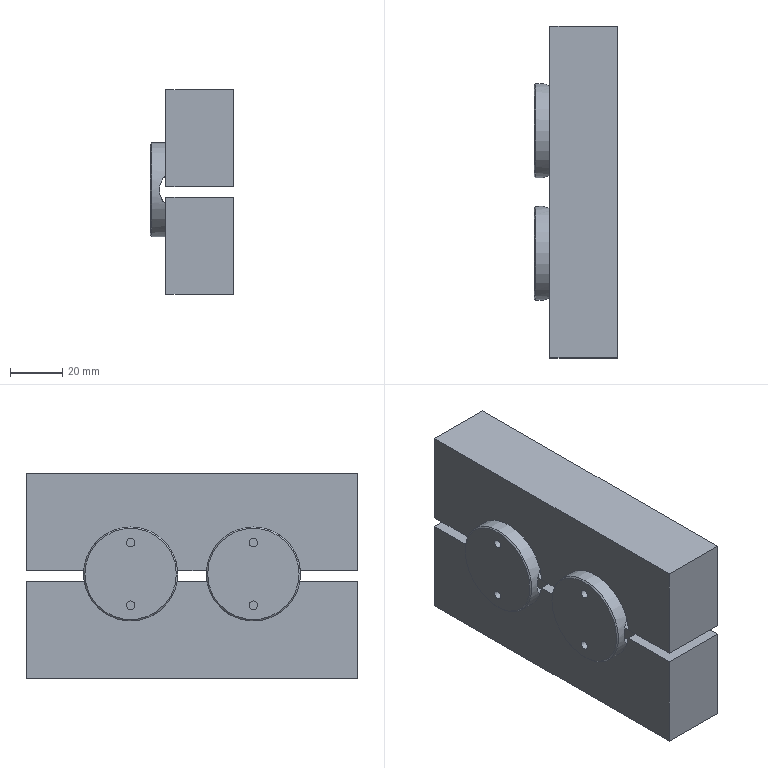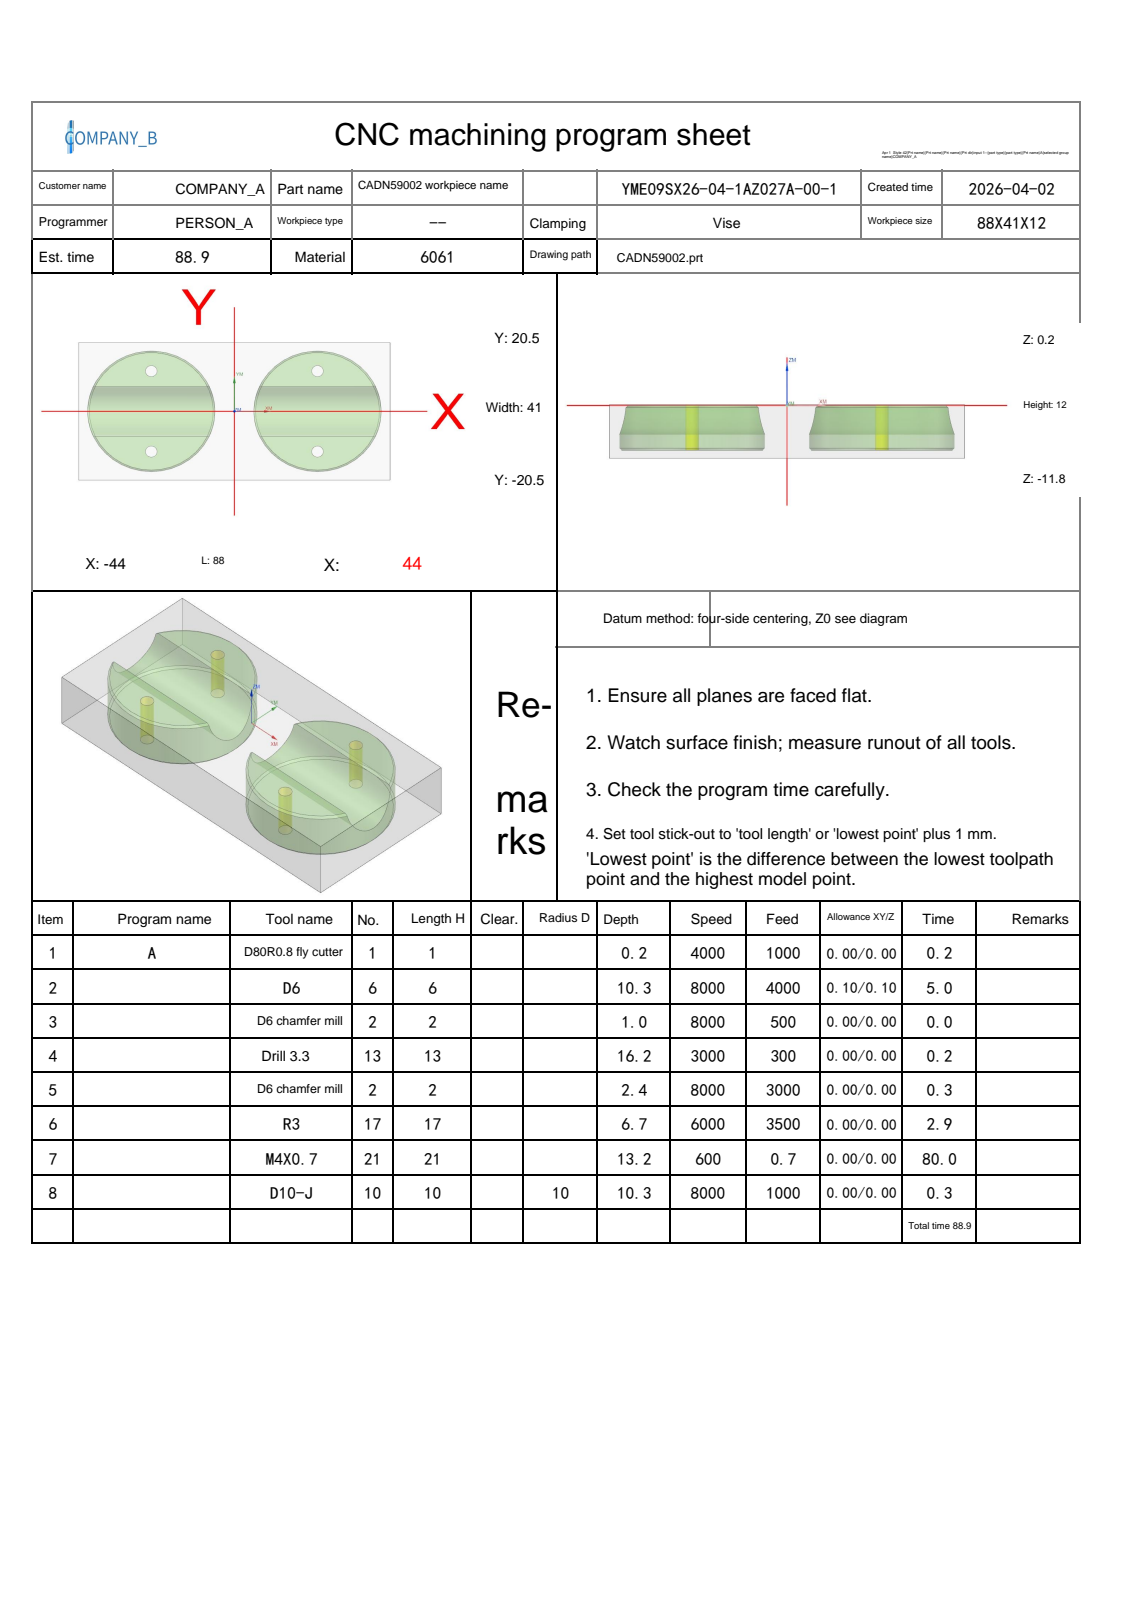NC program | NX | posted by the shop | part box 32 x 127 x 78.432 mm
Lines 6165 to 8369 of 8369:
N3 T02 M06
(D6 chamfer mill  D=6. R=0. H=02 ce=0.00 di=0.10)
G00 G90 G54 X-23.5 Y-12. M03 S8000
G43 H02 Z20.
M08
G98 G81 X-23.5 Y-12. Z-.8 R1. F500.
Y12.
X23.5 Y-12.
Y12.
G80
G00 Z20.
G91 G28 Z0.0
M05
M09
G91 G28 Z0.0
M01
N4 T13 M06
(drill 3.3 D=3.3 DR_a=118 H=13)
G00 G90 G54 X-23.5 Y-12. M03 S3000
G43 H13 Z20.
M08
G98 G83 X-23.5 Y-12. Z-15.991 R1. F300. Q2.
Y12.
X23.5 Y-12.
Y12.
G80
G00 Z20.
G91 G28 Z0.0
M05
M09
G91 G28 Z0.0
M01
N5 T02 M06
(D6 chamfer mill  D=6. R=0. H=02 ce=0.00 di=0.00)
G00 G90 G54 X7.369 Y-6.165 M03 S8000
G43 H02 Z20.
M08
Z2.927
G01 Z-1.499 F3000.
X7.657 Y-6.133
X23.5
X39.343
X39.631 Y-6.165
Z2.927
G00 Z20.
Y6.165
Z2.927
G01 Z-1.499
X39.343 Y6.133
X23.5
X7.657
X7.369 Y6.165
Z2.927
G00 Z20.
X-39.631 Y-6.165
Z2.927
G01 Z-1.499
X-39.343 Y-6.133
X-23.5
X-7.657
X-7.369 Y-6.165
Z2.927
G00 Z20.
Y6.165
Z2.927
G01 Z-1.499
X-7.657 Y6.133
X-23.5
X-39.343
X-39.631 Y6.165
Z2.927
G00 Z20.
G00 G90 X-23.5 Y-12. M03 S8000
Z20.
G98 G81 X-23.5 Y-12. Z-2.2 R3. F500.
Y12.
X23.5 Y-12.
Y12.
G80
G00 Z20.
G00 G90 X-5.262 Y-5.033 M03 S6500
Z20.
Z.3
G01 Z-1.2 F1500.
X-5.284 Y-5.071
X-5.301 Y-5.112
X-6.442 Y-7.662
X-6.452 Y-7.685
X-6.459 Y-7.7
X-6.472 Y-7.73
X-6.491 Y-7.772
X-6.503 Y-7.797
X-6.53 Y-7.856
G02 X-9.998 Y-12.938 I-16.97 J7.856
G01 X-10.106 Y-13.049
G02 X-14.986 Y-16.65 I-13.394 J13.049
X-15.531 Y-16.917 I-8.514 J16.65
X-16.05 Y-17.152 I-7.969 J16.917
X-16.645 Y-17.398 I-7.45 J17.152
X-18.14 Y-17.915 I-6.855 J17.398
X-18.931 Y-18.133 I-5.36 J17.915
G01 X-18.974 Y-18.144
G02 X-19.486 Y-18.264 I-4.526 J18.144
X-19.856 Y-18.342 I-4.014 J18.264
G01 X-19.991 Y-18.368
G02 X-23.5 Y-18.7 I-3.509 J18.368
X-28.05 Y-18.138 I0.0 J18.7
G01 X-28.085 Y-18.129
X-28.15 Y-18.113
X-28.271 Y-18.081
X-28.291 Y-18.076
G02 X-29.664 Y-17.655 I4.791 J18.076
G01 X-29.724 Y-17.634
G02 X-30.114 Y-17.491 I6.224 J17.634
X-30.371 Y-17.392 I6.614 J17.491
G01 X-30.411 Y-17.376
G02 X-31.138 Y-17.069 I6.911 J17.376
G01 X-31.185 Y-17.048
X-31.27 Y-17.01
X-31.308 Y-16.992
X-31.401 Y-16.949
X-31.49 Y-16.907
G02 X-40.436 Y-7.928 I7.99 J16.907
G01 X-40.456 Y-7.885
X-40.487 Y-7.819
X-40.51 Y-7.768
X-40.531 Y-7.723
X-40.548 Y-7.685
X-40.558 Y-7.662
X-40.568 Y-7.639
X-41.198 Y-6.233
X-41.699 Y-5.112
X-41.716 Y-5.071
X-41.738 Y-5.033
Z.3
G00 Z20.
Y5.033
Z.3
G01 Z-1.2
X-41.716 Y5.071
X-41.699 Y5.112
X-40.568 Y7.639
X-40.562 Y7.654
X-40.551 Y7.677
X-40.528 Y7.73
X-40.513 Y7.762
X-40.507 Y7.774
X-40.497 Y7.797
X-40.492 Y7.807
X-40.487 Y7.819
X-40.48 Y7.833
X-40.463 Y7.87
X-40.455 Y7.889
X-40.444 Y7.911
X-40.44 Y7.921
G02 X-40.329 Y8.154 I16.94 J-7.921
X-33.334 Y15.906 I16.829 J-8.154
X-33.121 Y16.035 I9.834 J-15.906
X-32.62 Y16.325 I9.621 J-16.035
G01 X-32.571 Y16.352
X-32.56 Y16.359
X-32.549 Y16.365
X-32.444 Y16.422
G02 X-32.105 Y16.602 I8.944 J-16.422
X-26.473 Y18.462 I8.605 J-16.602
G01 X-26.347 Y18.482
X-26.216 Y18.502
G02 X-25.978 Y18.535 I2.716 J-18.502
G01 X-25.933 Y18.541
X-25.902 Y18.545
G02 X-25.674 Y18.573 I2.402 J-18.545
G01 X-25.66 Y18.575
X-25.613 Y18.58
X-25.415 Y18.602
G02 X-25.014 Y18.639 I1.915 J-18.602
X-24.355 Y18.68 I1.514 J-18.639
G01 X-24.192 Y18.687
X-24.005 Y18.693
X-23.952 Y18.695
X-23.94
X-23.848 Y18.697
X-23.819
X-23.801 Y18.698
G02 X-23.5 Y18.7 I.301 J-18.698
X-22.885 Y18.69 I0.0 J-18.7
X-17.308 Y17.645 I-.615 J-18.69
X-15.815 Y17.048 I-6.192 J-17.645
G01 X-15.785 Y17.034
X-15.748 Y17.017
X-15.599 Y16.949
G02 X-14.745 Y16.524 I-7.901 J-16.949
X-14.015 Y16.116 I-8.755 J-16.524
G01 X-13.997 Y16.105
G02 X-13.493 Y15.797 I-9.503 J-16.105
X-13.265 Y15.65 I-10.007 J-15.797
G01 X-13.256 Y15.644
X-13.244 Y15.637
X-13.231 Y15.628
X-13.157 Y15.579
X-13.141 Y15.569
X-13.013 Y15.482
G02 X-6.57 Y7.942 I-10.487 J-15.482
G01 X-6.564 Y7.928
X-6.551 Y7.9
X-6.533 Y7.862
X-6.528 Y7.851
X-6.523 Y7.841
X-6.503 Y7.797
X-6.487 Y7.762
X-6.476 Y7.738
X-6.471 Y7.726
X-6.466 Y7.715
X-6.456 Y7.693
X-6.452 Y7.684
X-6.432 Y7.64
X-5.301 Y5.112
X-5.284 Y5.071
X-5.261 Y5.033
Z.3
G00 Z20.
X5.262
Z.3
G01 Z-1.2
X5.284 Y5.071
X5.301 Y5.112
X5.802 Y6.233
X6.432 Y7.639
X6.444 Y7.666
X6.449 Y7.677
X6.467 Y7.717
X6.484 Y7.756
X6.503 Y7.798
X6.517 Y7.827
X6.53 Y7.856
X6.539 Y7.876
X6.554 Y7.907
G02 X6.759 Y8.332 I16.946 J-7.907
X6.854 Y8.521 I16.741 J-8.332
G01 X6.876 Y8.563
X6.889 Y8.589
X6.929 Y8.665
G02 X7.564 Y9.784 I16.571 J-8.665
X7.738 Y10.062 I15.936 J-9.784
X8.021 Y10.493 I15.762 J-10.062
X23.5 Y18.7 I15.479 J-10.493
X32.987 Y16.115 I0.0 J-18.7
X33.233 Y15.967 I-9.487 J-16.115
X40.442 Y7.915 I-9.733 J-15.967
G01 X40.449 Y7.901
X40.453 Y7.892
X40.461 Y7.875
X40.468 Y7.861
X40.477 Y7.841
X40.483 Y7.826
X40.495 Y7.8
X40.504 Y7.782
X40.509 Y7.771
X40.536 Y7.712
X40.544 Y7.694
X40.568 Y7.639
X41.699 Y5.112
X41.716 Y5.071
X41.738 Y5.033
Z.3
G00 Z20.
Y-5.033
Z.3
G01 Z-1.2
X41.716 Y-5.071
X41.699 Y-5.112
X40.568 Y-7.639
X40.562 Y-7.655
X40.534 Y-7.715
X40.524 Y-7.739
X40.514 Y-7.76
X40.454 Y-7.89
X40.446 Y-7.907
X40.401 Y-8.003
X40.394 Y-8.018
X40.36 Y-8.089
X40.306 Y-8.2
X40.286 Y-8.242
G02 X40.021 Y-8.761 I-16.786 J8.242
X39.727 Y-9.293 I-16.521 J8.761
X25.965 Y-18.537 I-16.227 J9.293
G01 X25.931 Y-18.541
G02 X25.621 Y-18.579 I-2.431 J18.541
G01 X25.487 Y-18.594
X25.39 Y-18.604
X25.271 Y-18.616
X25.211 Y-18.622
G02 X23.5 Y-18.7 I-1.711 J18.622
X22.897 Y-18.69 I0.0 J18.7
X22.668 Y-18.681 I.603 J18.69
X22.382 Y-18.667 I.832 J18.681
X15.63 Y-16.963 I1.118 J18.667
X15.406 Y-16.858 I7.87 J16.963
X15.059 Y-16.687 I8.094 J16.858
X11.652 Y-14.468 I8.441 J16.687
G01 X11.582 Y-14.41
X11.536 Y-14.372
G02 X11.2 Y-14.086 I11.964 J14.372
X7.649 Y-9.922 I12.3 J14.086
X6.943 Y-8.693 I15.851 J9.922
X6.571 Y-7.943 I16.557 J8.693
G01 X6.551 Y-7.9
X6.544 Y-7.885
X6.481 Y-7.749
X6.432 Y-7.64
X5.301 Y-5.112
X5.284 Y-5.071
X5.261 Y-5.033
Z.3
G00 Z20.
G91 G28 Z0.0
M05
M09
G91 G28 Z0.0
M01
N6 T17 M06
(R3  D=6. R=3. H=17 ce=0.00 di=0.00)
G00 G90 G54 X41.596 Y-4.514 M03 S6000
G43 H17 Z20.
M08
Z2.989
G01 Z-2.299 F3500.
X39.597 Z-2.224
X39.476 Z-2.219
X39.348 Z-2.222
X37.885 Z-2.213
X36.422 Z-2.21
X17.099 Z-2.208
X9.602 Z-2.21
X7.884 Z-2.223
X7.651
X7.523 Z-2.221
X7.381 Z-2.226
X7.255 Y-4.5 Z-2.315
X7.385 Z-2.318
X7.462 Z-2.315
X7.71 Z-2.318
X8.97 Z-2.313
X9.801 Z-2.308
X36.278
X38.229 Z-2.311
X39.348 Z-2.318
X39.537 Z-2.313
X39.614 Z-2.316
X39.745 Z-2.314
X39.888 Y-4.486 Z-2.415
X39.821 Z-2.405
X39.598 Z-2.406
X39.348 Z-2.413
X37.885 Z-2.407
X9.568
X8.105 Z-2.413
X7.651 Z-2.414
X7.179 Z-2.405
X7.115 Z-2.414
X6.98 Y-4.472 Z-2.51
X7.085 Z-2.496
X7.163 Z-2.495
X7.233 Z-2.502
X7.382 Z-2.505
X7.651 Z-2.503
X9.114 Z-2.499
X9.602 Z-2.497
X38.373 Z-2.498
X39.348 Z-2.502
X39.573 Z-2.496
X39.836 Z-2.495
X39.915 Z-2.497
X40.026 Z-2.511
X40.164 Y-4.458 Z-2.607
X40.028 Z-2.589
X39.752 Z-2.584
X39.156 Z-2.589
X37.885 Z-2.586
X9.602
X7.651 Z-2.589
X7.438 Z-2.603
X7.333 Z-2.601
X7.163 Z-2.585
X6.972 Z-2.589
X6.845 Z-2.605
X6.769 Y-4.45 Z-2.659
X6.651 Y-4.444 Z-2.699
X6.676 Z-2.705
X6.858 Z-2.682
X7.163 Z-2.676
X7.325 Z-2.692
X7.448 Z-2.69
X7.651 Z-2.677
X11.54 Z-2.675
X38.373
X39.043 Z-2.677
X39.702 Z-2.674
X40.142 Z-2.682
X40.303 Z-2.703
X40.376 Y-4.432 Z-2.757
X40.381 Y-4.431 Z-2.764
X40.384 Y-4.429 Z-2.775
X40.339 Z-2.784
X39.836 Z-2.775
X39.649 Z-2.771
X7.651 Z-2.772
X7.586 Z-2.776
X7.377
X7.215 Z-2.78
X7.163 Z-2.775
X6.734 Z-2.783
X6.676 Z-2.79
X6.612 Z-2.774
X6.594 Y-4.411 Z-2.87
X6.632 Z-2.88
X6.851 Z-2.879
X7.375 Z-2.869
X39.624
X40.148 Z-2.879
X40.368 Z-2.88
X40.407 Z-2.87
X40.434 Y-4.39 Z-2.973
X40.324 Z-2.971
X39.827
X39.627 Z-2.966
X7.373
X7.142 Z-2.971
X6.676 Z-2.97
X6.568 Z-2.973
X6.543 Y-4.369 Z-3.066
X6.676 Z-3.063
X7.314 Z-3.065
X7.37 Z-3.064
X39.629
X39.836 Z-3.065
X40.324 Z-3.062
X40.458 Z-3.065
X40.482 Y-4.345 Z-3.159
X40.324 Z-3.156
X39.836 Z-3.159
X7.163
X6.676 Z-3.156
X6.518 Z-3.16
X6.5 Y-4.329 Z-3.225
X6.494 Y-4.321 Z-3.251
X6.552 Z-3.252
X6.593 Z-3.244
X6.676 Z-3.242
X7.163 Z-3.246
X39.836
X40.324 Z-3.242
X40.406 Z-3.244
X40.447 Z-3.252
X40.507 Z-3.253
X40.53 Y-4.293 Z-3.343
X40.324 Z-3.337
X39.836 Z-3.34
X7.163
X6.514 Z-3.336
X6.471 Z-3.338
X6.447 Y-4.265 Z-3.431
X6.599 Z-3.423
X7.163 Z-3.427
X39.836
X40.324 Z-3.424
X40.554 Z-3.435
X40.577 Y-4.236 Z-3.523
X40.324 Z-3.511
X39.836 Z-3.514
X7.163
X6.66 Z-3.512
X6.423 Z-3.523
X6.398 Y-4.199 Z-3.613
X6.511 Z-3.607
X6.676 Z-3.604
X7.163 Z-3.607
X39.836
X40.324 Z-3.604
X40.488 Z-3.607
X40.601 Z-3.613
X40.627 Y-4.162 Z-3.702
X40.324 Z-3.696
X39.836 Z-3.698
X6.989 Z-3.697
X6.676 Z-3.696
X6.374 Z-3.702
X6.347 Y-4.127 Z-3.791
X6.676 Z-3.785
X8.184 Z-3.787
X39.836
X40.324 Z-3.785
X40.655 Z-3.791
X40.683 Y-4.087 Z-3.878
X40.453 Z-3.874
X7.034 Z-3.875
X6.547 Z-3.874
X6.319 Z-3.878
X6.29 Y-4.045 Z-3.965
X6.676 Z-3.962
X40.62 Z-3.963
X40.711 Z-3.965
X40.739 Y-4.004 Z-4.051
X6.262
X6.233 Y-3.957 Z-4.137
X40.768 Z-4.136
X40.796 Y-3.911 Z-4.22
X6.204
X6.173 Y-3.864 Z-4.303
X40.324
X40.827
X40.859 Y-3.814 Z-4.384
X40.811 Z-4.38
X39.279 Z-4.382
X6.438 Z-4.381
X6.188
X6.142 Z-4.384
X6.124 Y-3.787 Z-4.428
X6.109 Y-3.761 Z-4.466
X40.301 Z-4.467
X40.891 Z-4.466
X40.923 Y-3.706 Z-4.546
X40.811 Z-4.545
X40.324 Z-4.547
X6.676
X6.077
X6.045 Y-3.652 Z-4.624
X6.188 Z-4.623
X7.727 Z-4.625
X40.324
X40.811 Z-4.623
X40.955 Z-4.624
X40.966 Y-3.634 Z-4.65
X40.988 Y-3.595 Z-4.7
X40.811 Z-4.698
X38.974 Z-4.7
X30.083
X29.924 Z-4.702
X22.928
X22.768 Z-4.699
X6.676 Z-4.7
X6.148 Z-4.698
X6.012 Z-4.7
X5.979 Y-3.536 Z-4.773
X22.768
X23.164 Z-4.78
X29.687
X30.083 Z-4.774
X40.522 Z-4.773
X41.021 Z-4.774
X41.054 Y-3.476 Z-4.848
X30.083
X29.743 Z-4.853
X23.108
X22.768 Z-4.847
X5.945 Z-4.848
X5.911 Y-3.414 Z-4.927
X5.967 Z-4.925
X22.768 Z-4.924
X22.859 Z-4.926
X29.992 Z-4.927
X30.083 Z-4.926
X41.055 Z-4.925
X41.089 Z-4.927
X41.102 Y-3.392 Z-4.956
X41.122 Y-3.352 Z-4.997
X14.234 Z-4.996
X5.878 Z-4.997
X5.844 Y-3.287 Z-5.066
X41.156
X41.19 Y-3.222 Z-5.135
X5.81
X5.776 Y-3.155 Z-5.206
X41.224
X41.259 Y-3.083 Z-5.273
X40.946 Z-5.272
X40.593 Z-5.274
X40.458 Z-5.273
X6.541
X6.188 Z-5.274
X6.053 Z-5.272
X5.741 Z-5.273
X5.706 Y-3.01 Z-5.339
X5.907 Z-5.338
X6.188 Z-5.341
X6.395 Z-5.339
X40.605
X40.886 Z-5.341
X41.092 Z-5.338
X41.294
X41.328 Y-2.939 Z-5.403
X5.829
X5.672
X5.658 Y-2.907 Z-5.433
X5.64 Y-2.867 Z-5.465
X5.7 Z-5.463
X41.299
X41.36 Z-5.465
X41.392 Y-2.794 Z-5.525
X41.299 Z-5.522
X5.7 Z-5.521
X5.608 Z-5.525
X5.575 Y-2.719 Z-5.586
X5.7 Z-5.581
X41.299
X41.425 Z-5.586
X41.449 Y-2.665 Z-5.631
X41.458 Y-2.641 Z-5.646
X41.323 Z-5.64
X5.676
X5.543 Z-5.646
X5.512 Y-2.56 Z-5.7
X5.594 Z-5.696
X41.405
X41.489 Z-5.7
X41.521 Y-2.478 Z-5.753
X41.487 Z-5.751
X5.513
X5.481 Z-5.753
X5.45 Y-2.398 Z-5.806
X5.7 Z-5.804
X41.517
X41.552 Z-5.806
X41.583 Y-2.317 Z-5.859
X41.437 Z-5.853
X5.563
X5.419 Z-5.859
X5.389 Y-2.234 Z-5.907
X5.592 Z-5.905
X5.646 Z-5.903
X41.353 Z-5.902
X41.408 Z-5.905
X41.611 Z-5.907
X41.628 Y-2.18 Z-5.938
X41.637 Y-2.148 Z-5.954
X41.233 Z-5.952
X5.635
X5.361 Z-5.954
X5.336 Y-2.06 Z-5.999
X27.935 Z-5.996
X41.663 Z-5.999
X41.688 Y-1.973 Z-6.042
X20.504 Z-6.039
X5.311 Z-6.043
X5.301 Y-1.938 Z-6.06
X5.287 Y-1.885 Z-6.083
X26.989 Z-6.081
X41.712 Z-6.083
X41.737 Y-1.796 Z-6.121
X12.402
X5.262 Z-6.122
X5.238 Y-1.706 Z-6.16
X41.762
X41.783 Y-1.613 Z-6.196
X41.145 Z-6.199
X40.811 Z-6.197
X6.188
X5.547 Z-6.199
X5.217 Z-6.196
X5.196 Y-1.521 Z-6.231
X5.918 Z-6.233
X6.188 Z-6.231
X40.811
X41.299 Z-6.233
X41.804 Z-6.231
X41.824 Y-1.429 Z-6.264
X5.176
X5.155 Y-1.336 Z-6.294
X5.213 Z-6.293
X20.58
X20.818 Z-6.289
X21.424
X21.543 Z-6.293
X41.787
X41.845 Z-6.294
X41.865 Y-1.242 Z-6.323
X21.731 Z-6.322
X21.518 Z-6.316
X20.818
X20.391 Z-6.322
X7.407 Z-6.323
X5.135
X5.119 Y-1.146 Z-6.349
X20.462 Z-6.348
X20.818 Z-6.343
X21.615
X21.793 Z-6.348
X41.881 Z-6.349
X41.896 Y-1.05 Z-6.373
X26.426 Z-6.372
X21.793
X21.711 Z-6.37
X20.818
X20.655 Z-6.372
X5.104 Z-6.373
X5.089 Y-.954 Z-6.397
X27.157 Z-6.394
X41.787 Z-6.395
X41.911 Z-6.396
X41.925 Y-.857 Z-6.415
X23.275 Z-6.414
X5.075 Z-6.415
X5.06 Y-.759 Z-6.431
X5.213 Z-6.433
X41.819
X41.94 Z-6.431
X41.944 Y-.733 Z-6.435
X41.949 Y-.661 Z-6.447
X41.787 Z-6.449
X5.146
X5.051 Z-6.447
X5.043 Y-.562 Z-6.463
X41.957
X41.965 Y-.463 Z-6.475
X5.035
X5.027 Y-.364 Z-6.485
X5.213 Z-6.483
X41.909
X41.973 Z-6.485
X41.981 Y-.265 Z-6.496
X41.81 Z-6.491
X5.19
X5.019 Z-6.496
X5.017 Y-.242 Z-6.498
Y-.165
X5.213 Z-6.495
X41.864
X41.983 Z-6.498
Y-.065
X5.017
Y.035
X41.983
Y.135 Z-6.497
X41.895 Z-6.495
X5.105 Z-6.496
X5.016 Z-6.498
Y.235
X5.205 Z-6.493
X41.794 Z-6.492
X41.983 Z-6.497
X41.976 Y.334 Z-6.487
X41.787 Z-6.484
X5.12 Z-6.485
X5.023 Z-6.488
X5.031 Y.434 Z-6.477
X15.941 Z-6.474
X29.412 Z-6.477
X41.969 Z-6.476
X41.965 Y.485 Z-6.472
X41.961 Y.533 Z-6.466
X18.867 Z-6.464
X14.966 Z-6.461
X14.869 Z-6.463
X5.039 Z-6.466
X5.046 Y.631 Z-6.451
X6.92 Z-6.452
X14.67 Z-6.45
X14.966 Z-6.445
X18.719 Z-6.446
X18.867 Z-6.449
X32.521 Z-6.45
X41.883 Z-6.452
X41.953 Z-6.45
X41.946 Y.73 Z-6.435
X41.787 Z-6.438
X24.956 Z-6.432
X18.861 Z-6.434
X18.62 Z-6.43
X14.966 Z-6.429
X14.478 Z-6.437
X5.694 Z-6.438
X5.21
X5.054 Z-6.435
X5.068 Y.828 Z-6.42
X14.682 Z-6.418
X14.966 Z-6.413
X18.521 Z-6.414
X18.663 Z-6.416
X34.02 Z-6.418
X41.931 Z-6.42
X41.917 Y.926 Z-6.403
X14.966 Z-6.397
X5.299 Z-6.402
X5.083 Z-6.403
X5.089 Y.969 Z-6.395
X5.097 Y1.024 Z-6.381
X17.16 Z-6.378
X23.256 Z-6.379
X23.311 Z-6.377
X41.902 Z-6.381
X41.888 Y1.12 Z-6.356
X29.899 Z-6.354
X29.595 Z-6.351
X23.408
X23.256 Z-6.355
X5.112 Z-6.356
X5.126 Y1.216 Z-6.331
X23.266
X23.505 Z-6.324
X29.595 Z-6.325
X30.073 Z-6.329
X41.792 Z-6.332
X41.874 Z-6.33
X41.853 Y1.312 Z-6.303
X41.787 Z-6.302
X29.881 Z-6.3
X29.595 Z-6.298
X23.601 Z-6.297
X23.458 Z-6.302
X5.213
X5.147 Z-6.303
X5.168 Y1.407 Z-6.273
X23.65 Z-6.272
X23.697 Z-6.271
X41.832 Z-6.273
X41.821 Y1.454 Z-6.259
X41.81 Y1.502 Z-6.24
X5.407 Z-6.241
X5.19 Z-6.24
X5.211 Y1.595 Z-6.204
X5.783 Z-6.207
X5.985 Z-6.204
X40.811
X41.378 Z-6.206
X41.789 Z-6.204
X41.768 Y1.688 Z-6.168
X5.232
X5.256 Y1.779 Z-6.128
X41.744
X41.718 Y1.871 Z-6.088
X5.282
X5.307 Y1.962 Z-6.047
X41.692 Z-6.046
X41.666 Y2.051 Z-6.002
X5.333
X5.359 Y2.14 Z-5.957
X5.7 Z-5.955
X41.381
X41.64 Z-5.957
X41.622 Y2.201 Z-5.925
X41.613 Y2.227 Z-5.91
X41.299 Z-5.906
X5.7
X5.385 Z-5.91
X5.417 Y2.313 Z-5.861
X5.7 Z-5.855
X41.299
X41.585 Z-5.861
X41.553 Y2.399 Z-5.81
X41.299 Z-5.804
X5.7
X5.45 Z-5.81
X5.459 Y2.423 Z-5.795
X5.482 Y2.482 Z-5.754
X5.7 Z-5.749
X41.299
X41.52 Z-5.754
X41.487 Y2.564 Z-5.696
X41.299 Z-5.692
X5.7
X5.514 Z-5.696
X5.546 Y2.646 Z-5.641
X5.7 Z-5.635
X41.336 Z-5.636
X41.455 Z-5.641
X41.448 Y2.665 Z-5.629
X41.422 Y2.726 Z-5.579
X41.299 Z-5.574
X5.7
X5.579 Z-5.579
X5.613 Y2.804 Z-5.515
X5.7 Z-5.512
X41.299
X41.387 Z-5.515
X41.353 Y2.883 Z-5.452
X41.299 Z-5.451
X5.7 Z-5.45
X5.647 Z-5.452
X5.67 Y2.935 Z-5.407
X5.681 Y2.958 Z-5.386
X5.803 Z-5.385
X6.188 Z-5.387
X6.29 Z-5.386
X40.709
X40.811 Z-5.388
X41.095 Z-5.387
X41.299 Z-5.385
X41.319 Z-5.386
X41.284 Y3.031 Z-5.319
X41.049
X40.8 Z-5.323
X40.562 Z-5.32
X6.438
X6.188 Z-5.323
X5.95 Z-5.319
X5.716
X5.751 Y3.104 Z-5.253
X6.097
X6.493 Z-5.255
X6.584 Z-5.254
X40.415
X40.811 Z-5.255
X40.903 Z-5.253
X41.249
X41.228 Y3.15 Z-5.213
X41.215 Y3.175 Z-5.186
X5.785
X5.82 Y3.243 Z-5.115
X5.999
X6.188 Z-5.111
X40.811 Y3.244 Z-5.112
X41. Z-5.115
X41.18
X41.145 Y3.312 Z-5.044
X40.811 Z-5.038
X6.188
X5.855 Z-5.044
X5.891 Y3.38 Z-4.971
X6.188 Z-4.965
X10.882 Z-4.967
X40.324
X40.811 Z-4.965
X41.109 Z-4.97
X41.074 Y3.443 Z-4.893
X40.811 Z-4.889
X30.571
X30.365 Z-4.892
X16.147
X15.941 Z-4.89
X6.676
X6.188 Z-4.889
X5.926 Z-4.893
X5.961 Y3.505 Z-4.816
X6.188 Z-4.811
X15.941 Z-4.813
X16.397 Z-4.818
X30.114
X30.571 Z-4.811
X40.811 Z-4.812
X41.039 Z-4.816
X41.005 Y3.566 Z-4.742
X40.949 Z-4.739
X40.811 Z-4.736
X30.571 Z-4.734
X30.296 Z-4.738
X16.216 Z-4.74
X15.941 Z-4.737
X6.188 Z-4.736
X6.051 Z-4.739
X5.994 Z-4.742
X6.027 Y3.626 Z-4.67
X6.188 Z-4.661
X18.404 Z-4.662
X31.042 Z-4.658
X40.828 Z-4.662
X40.973 Z-4.67
X40.94 Y3.682 Z-4.59
X40.811 Z-4.583
X24.04 Z-4.582
X22.472
X22.281 Z-4.577
X16.429 Z-4.579
X16.238 Z-4.583
X6.188
X6.061 Z-4.59
X6.092 Y3.736 Z-4.51
X6.188 Z-4.504
X16.017 Z-4.503
X16.429 Z-4.496
X22.281 Z-4.494
X22.692 Z-4.505
X40.811 Z-4.504
X40.908 Z-4.51
X40.897 Y3.755 Z-4.485
X40.875 Y3.79 Z-4.425
X40.811 Z-4.42
X22.628 Z-4.421
X22.281 Z-4.412
X16.429 Z-4.413
X16.082 Z-4.42
X6.188
X6.125 Z-4.425
X6.159 Y3.842 Z-4.337
X6.188 Z-4.335
X9.114 Z-4.336
X16.292
X16.429 Z-4.333
X22.281
X22.417 Z-4.337
X40.46 Z-4.336
X40.811 Z-4.335
X40.842 Z-4.337
X40.809 Y3.893 Z-4.249
X37.4 Z-4.251
X6.676 Z-4.25
X6.192 Z-4.249
X6.222 Y3.941 Z-4.162
X40.324 Z-4.163
X40.778 Z-4.162
X40.749 Y3.989 Z-4.076
X6.252
X6.282 Y4.033 Z-3.987
X7.02 Z-3.986
X39.979
X40.719 Z-3.987
X40.69 Y4.076 Z-3.899
X40.496 Z-3.895
X30.647 Z-3.896
X7.163
X6.504 Z-3.895
X6.311 Z-3.898
X6.34 Y4.119 Z-3.81
X6.674 Z-3.804
X7.163 Z-3.806
X39.835
X40.324 Z-3.804
X40.661 Z-3.81
X40.632 Y4.156 Z-3.717
X40.324 Z-3.712
X39.836 Z-3.714
X32.034
X31.734 Z-3.718
X31.358
X31.058 Z-3.714
X7.163
X6.676 Z-3.712
X6.369 Z-3.717
X6.395 Y4.193 Z-3.627
X6.487 Z-3.622
X6.676 Z-3.619
X7.163 Z-3.621
X31.058
X31.436 Z-3.627
X31.656
X32.034 Z-3.621
X39.836
X40.324 Z-3.619
X40.512 Z-3.622
X40.605 Z-3.627
X40.581 Y4.229 Z-3.541
X40.324 Z-3.53
X39.836 Z-3.532
X32.034
X31.149 Z-3.534
X31.058 Z-3.533
X7.163
X6.63 Z-3.531
X6.419 Z-3.541
X6.426 Y4.24 Z-3.514
X6.443 Y4.26 Z-3.453
X6.676 Z-3.442
X7.651 Z-3.444
X23.096 Z-3.441
X31.386 Z-3.443
X31.466 Z-3.439
X36.422
X36.582 Z-3.444
X39.836 Z-3.445
X40.324 Z-3.442
X40.558 Z-3.454
X40.535 Y4.288 Z-3.366
X40.426 Z-3.363
X40.324 Z-3.359
X39.836 Z-3.361
X36.808
X36.422 Z-3.347
X31.353
X31.161 Z-3.357
X20.33 Z-3.351
X7.163 Z-3.36
X6.676 Z-3.359
X6.573 Z-3.363
X6.466 Z-3.366
X6.489 Y4.315 Z-3.277
X6.586 Z-3.275
X6.616 Z-3.269
X6.676 Z-3.267
X7.163 Z-3.269
X21.425 Z-3.26
X31.058 Z-3.265
X31.242 Z-3.256
X36.422
X36.79 Z-3.269
X39.836
X40.324 Z-3.267
X40.383 Z-3.269
X40.413 Z-3.275
X40.511 Z-3.277
X40.499 Y4.33 Z-3.231
X40.487 Y4.341 Z-3.18
X40.324 Z-3.176
X39.836 Z-3.178
X36.584
X36.422 Z-3.172
X31.139
X31.058 Z-3.176
X17.892 Z-3.174
X7.163 Z-3.178
X6.676 Z-3.176
X6.514 Z-3.18
X6.539 Y4.366 Z-3.084
X6.76 Z-3.08
X7.37 Z-3.081
X39.836 Z-3.082
X40.324 Z-3.08
X40.462 Z-3.084
X40.438 Y4.387 Z-2.99
X40.324 Z-2.988
X39.805 Z-2.986
X39.627 Z-2.983
X7.372
X7.194 Z-2.986
X6.676 Z-2.988
X6.562 Z-2.991
X6.583 Y4.407 Z-2.892
X6.616 Z-2.899
X7.163 Z-2.892
X7.375 Z-2.888
X39.625
X40.083 Z-2.896
X40.384 Z-2.899
X40.413 Z-2.892
X40.39 Y4.425 Z-2.797
X40.324 Z-2.812
X40.297 Z-2.809
X39.836 Z-2.801
X39.813 Z-2.803
X39.623 Z-2.799
X39.378
X39.348 Z-2.797
X7.365 Z-2.796
X6.687 Z-2.809
X6.657 Z-2.807
X6.605 Z-2.797
X6.622 Y4.44 Z-2.716
X6.662 Z-2.724
X6.69 Z-2.725
X6.825 Z-2.708
X7.311 Z-2.699
X8.139 Z-2.701
X37.398 Z-2.7
X39.348 Z-2.702
X39.515 Z-2.712
X39.703 Z-2.714
X39.836 Z-2.702
X40.174 Z-2.708
X40.296 Z-2.723
X40.162 Y4.456 Z-2.621
X40.05 Z-2.607
X39.836 Z-2.603
X39.646 Z-2.621
X39.587 Z-2.622
X39.348 Z-2.607
X36.476 Z-2.603
X8.626 Y4.455 Z-2.604
X7.866 Z-2.606
X7.257 Z-2.601
X6.949 Z-2.607
X6.805 Z-2.626
X6.945 Y4.47 Z-2.529
X7.063 Z-2.513
X7.207 Z-2.511
X7.438 Z-2.512
X7.651 Z-2.518
X9.114 Z-2.513
X37.398
X38.861 Z-2.518
X39.348
X39.618 Z-2.522
X39.747 Z-2.52
X39.836 Z-2.511
X39.936 Z-2.513
X40.033 Z-2.525
X39.897 Y4.484 Z-2.428
X39.829 Z-2.419
X39.348 Z-2.428
X38.367 Z-2.426
X37.376 Z-2.422
X9.108
X7.651 Z-2.428
X7.38 Z-2.421
X7.17 Z-2.419
X7.088 Z-2.431
X7.235 Y4.498 Z-2.328
X7.385 Z-2.329
X7.452 Z-2.327
X7.651 Z-2.333
X9.114 Z-2.325
X15.945 Z-2.322
X37.398 Z-2.324
X38.987 Z-2.333
X39.348
X39.547 Z-2.329
X39.614 Z-2.332
X39.759 Z-2.329
X39.634 Y4.512 Z-2.24
X39.486 Z-2.235
X39.348 Z-2.238
X38.61 Z-2.235
X37.16 Z-2.225
X25.088 Z-2.223
X10.326 Z-2.225
X9.602 Z-2.226
X8.863 Z-2.229
X7.651 Z-2.237
X7.513 Z-2.234
X7.382 Z-2.239
X7.489 Y4.518 Z-2.192
X7.563 Y4.522 Z-2.166
X7.651 Y4.524 Z-2.153
X7.799 Z-2.149
X9.253 Y4.525 Z-2.131
X9.95 Z-2.127
X17.97 Z-2.124
X35.587 Z-2.126
X37.398 Z-2.128
X37.979 Z-2.133
X39.979 Z-2.152
Z2.989
G00 Z20.
X-41.593 Y4.514
Z2.989
G01 Z-2.296
X-39.595 Z-2.22
X-39.475 Z-2.215
X-39.349 Z-2.219
X-37.886 Z-2.209
X-36.423 Z-2.206
X-17.335
X-9.602 Z-2.209
X-7.883 Z-2.222
X-7.652
X-7.524 Z-2.22
X-7.383 Z-2.225
X-7.256 Y4.5 Z-2.314
X-7.386 Z-2.317
X-7.463 Z-2.314
X-7.652 Z-2.317
X-8.482 Z-2.315
X-9.747 Z-2.307
X-36.275 Z-2.304
X-38.226 Y4.501 Z-2.307
X-39.349 Z-2.314
X-39.536 Z-2.309
X-39.615 Z-2.312
X-39.739 Z-2.311
X-39.882 Y4.487 Z-2.411
X-39.819 Z-2.401
X-39.597 Z-2.403
X-39.349 Z-2.409
X-37.886 Z-2.403
X-9.568 Y4.486 Z-2.405
X-8.105 Z-2.412
X-7.652
X-7.18 Z-2.404
X-7.114 Z-2.413
X-6.977 Y4.472 Z-2.509
X-7.086 Z-2.495
X-7.164 Z-2.494
X-7.234 Z-2.501
X-7.383 Z-2.504
X-7.652 Z-2.502
X-9.193 Z-2.498
X-9.602 Z-2.496
X-38.299 Y4.473 Z-2.495
X-39.349 Z-2.499
X-39.618 Z-2.493
X-39.837 Z-2.492
X-39.912 Z-2.493
X-40.02 Z-2.507
X-40.159 Y4.459 Z-2.603
X-40.025 Z-2.585
X-39.755 Z-2.58
X-39.514 Z-2.582
X-39.349 Z-2.586
X-37.886 Z-2.582
X-9.602 Y4.458 Z-2.585
X-8.139 Z-2.589
X-7.652
X-7.439 Z-2.602
X-7.334 Z-2.6
X-7.164 Z-2.584
X-6.973 Z-2.588
X-6.839 Z-2.605
X-6.711 Y4.448 Z-2.676
X-6.893 Z-2.653
X-7.164 Z-2.648
X-7.356 Y4.449 Z-2.666
X-7.41
X-7.652 Z-2.65
X-10.307 Z-2.647
X-38.374 Z-2.645
X-39.349 Z-2.647
X-39.47 Z-2.644
X-39.72 Z-2.643
X-40.104 Z-2.65
X-40.258 Z-2.671
X-40.324 Y4.442 Z-2.719
X-40.356 Y4.436 Z-2.743
X-40.324 Z-2.75
X-40.207 Z-2.734
X-39.675 Z-2.724
X-39.413 Z-2.725
X-39.349 Z-2.726
X-30.815
X-8.253 Z-2.729
X-7.652
X-7.525 Z-2.737
X-7.378
X-7.265 Z-2.74
X-7.164 Z-2.73
X-6.79 Z-2.737
X-6.692 Z-2.749
X-6.661 Z-2.747
X-6.619 Z-2.738
X-6.603 Y4.42 Z-2.821
X-6.67 Z-2.837
X-7.377 Z-2.824
X-39.624 Y4.421 Z-2.822
X-40.328 Z-2.835
X-40.395 Z-2.82
X-40.422 Y4.4 Z-2.927
X-40.411 Z-2.93
X-40.324 Z-2.928
X-39.977 Z-2.926
X-39.626 Z-2.92
X-7.374 Z-2.922
X-7.03 Z-2.928
X-6.674 Z-2.929
X-6.588 Z-2.931
X-6.58 Z-2.93
X-6.554 Y4.379 Z-3.025
X-6.676 Z-3.022
X-7.247 Z-3.021
X-7.372 Z-3.019
X-39.629 Y4.38 Z-3.018
X-39.837 Z-3.02
X-40.324
X-40.446 Z-3.023
X-40.47 Y4.358 Z-3.117
X-40.324 Z-3.113
X-39.837 Z-3.115
X-7.14 Z-3.117
X-6.676 Z-3.115
X-6.53 Z-3.118
X-6.506 Y4.334 Z-3.212
X-6.543 Z-3.205
X-6.676 Z-3.202
X-7.164 Z-3.204
X-10.357
X-10.578 Z-3.196
X-15.454
X-15.674 Z-3.201
X-28.402 Z-3.198
X-39.837 Z-3.202
X-40.324 Z-3.2
X-40.46 Z-3.204
X-40.494 Z-3.211
X-40.505 Y4.323 Z-3.253
X-40.518 Y4.308 Z-3.301
X-40.369 Z-3.298
X-40.354 Z-3.295
X-38.352
X-26.67 Z-3.286
X-17.484 Y4.307 Z-3.291
X-15.885 Z-3.293
X-15.454 Z-3.282
X-10.578
X-10.146 Z-3.298
X-7.164
X-6.649 Z-3.296
X-6.635 Z-3.299
X-6.483 Z-3.303
X-6.459 Y4.279 Z-3.395
X-6.676 Z-3.386
X-7.164 Z-3.388
X-10.265
X-10.578 Z-3.376
X-15.454
X-15.767 Z-3.384
X-26.67 Z-3.379
X-40.009 Z-3.386
X-40.324 Z-3.384
X-40.542 Z-3.394
X-40.566 Y4.25 Z-3.483
X-40.324 Z-3.472
X-39.837 Z-3.474
X-19.395 Z-3.473
X-15.532 Z-3.474
X-15.454 Z-3.472
X-10.578
X-10.5 Z-3.475
X-7.164
X-6.676 Z-3.473
X-6.434 Z-3.485
X-6.427 Y4.24 Z-3.514
X-6.41 Y4.216 Z-3.571
X-6.58 Z-3.563
X-6.676 Z-3.561
X-7.164 Z-3.564
X-14.966 Z-3.563
X-15.157 Z-3.566
X-15.751
X-15.942 Z-3.563
X-39.837
X-40.324 Z-3.56
X-40.419 Z-3.562
X-40.589 Z-3.57
X-40.614 Y4.181 Z-3.656
X-40.562 Z-3.654
X-40.324 Z-3.649
X-39.837 Z-3.652
X-15.942
X-15.444 Z-3.66
X-14.966 Z-3.652
X-6.916 Y4.18 Z-3.651
X-6.676 Z-3.65
X-6.437 Z-3.655
X-6.386 Z-3.657
X-6.361 Y4.144 Z-3.746
X-6.676 Z-3.741
X-7.164 Z-3.743
X-14.966 Z-3.742
X-15.173 Z-3.746
X-15.735
X-15.942 Z-3.743
X-39.837 Y4.145 Z-3.742
X-40.324 Z-3.74
X-40.641 Z-3.745
X-40.661 Y4.119 Z-3.811
X-40.669 Y4.107 Z-3.834
X-40.279 Z-3.829
X-39.837 Z-3.83
X-7.164 Z-3.831
X-6.629 Z-3.829
X-6.332 Z-3.835
X-6.303 Y4.065 Z-3.921
X-6.461 Z-3.918
X-40.11 Y4.066 Z-3.917
X-40.538
X-40.697 Z-3.92
X-40.726 Y4.024 Z-4.006
X-6.275 Y4.023 Z-4.007
X-6.257 Y3.998 Z-4.061
X-6.246 Y3.98 Z-4.092
X-40.754 Y3.981
X-40.782 Y3.934 Z-4.176
X-6.676 Z-4.177
X-6.218 Z-4.176
X-6.188 Y3.887 Z-4.26
X-9.206 Z-4.261
X-40.324 Y3.888 Z-4.26
X-40.812 Z-4.259
X-40.844 Y3.838 Z-4.344
X-40.812 Z-4.342
X-37.154 Z-4.343
X-30.725
X-30.571 Z-4.34
X-24.719 Z-4.339
X-24.565 Z-4.343
X-6.521
X-6.189 Z-4.342
X-6.156 Z-4.345
X-6.125 Y3.789 Z-4.427
X-6.189 Z-4.421
X-24.37 Y3.79 Z-4.422
X-24.719 Z-4.413
X-30.571 Z-4.414
X-30.92 Z-4.42
X-40.812 Z-4.421
X-40.875 Z-4.426
X-40.897 Y3.755 Z-4.485
X-40.906 Y3.739 Z-4.506
X-40.812 Z-4.5
X-30.994 Z-4.499
X-30.571 Z-4.491
X-24.719 Z-4.49
X-24.297 Z-4.501
X-6.189
X-6.094 Z-4.507
X-6.062 Y3.685 Z-4.585
X-6.189 Z-4.578
X-23.154 Z-4.577
X-24.514
X-24.719 Z-4.572
X-30.571 Z-4.574
X-30.777 Z-4.578
X-40.812 Z-4.577
X-40.937 Z-4.584
X-40.97 Y3.63 Z-4.664
X-40.804 Z-4.656
X-28.483
X-16.429 Z-4.653
X-6.18 Z-4.657
X-6.029 Z-4.665
X-5.996 Y3.57 Z-4.737
X-6.059 Z-4.734
X-6.189 Z-4.731
X-16.429 Z-4.729
X-16.688 Z-4.733
X-30.801 Z-4.735
X-31.059 Z-4.732
X-40.812 Z-4.731
X-40.941 Z-4.733
X-41.003 Z-4.737
X-41.036 Y3.51 Z-4.81
X-40.812 Z-4.806
X-31.059 Z-4.807
X-30.585 Z-4.812
X-16.902 Y3.509 Z-4.813
X-16.429 Z-4.805
X-6.189 Z-4.806
X-5.963 Z-4.81
X-5.928 Y3.447 Z-4.888
X-6.189 Z-4.884
X-16.429
X-16.653 Z-4.887
X-30.835 Y3.448
X-31.059 Z-4.884
X-40.324
X-40.812 Z-4.883
X-41.071 Z-4.888
X-41.105 Y3.387 Z-4.963
X-40.812 Z-4.957
X-37.16 Z-4.959
X-6.666
X-6.189 Z-4.958
X-5.894 Z-4.963
X-5.861 Y3.323 Z-5.032
X-6.189 Z-5.026
X-40.812
X-41.139 Z-5.032
X-41.174 Y3.255 Z-5.103
X-41.024
X-40.812 Z-5.099
X-6.189 Z-5.1
X-5.977 Z-5.103
X-5.826
X-5.791 Y3.187 Z-5.174
X-6.676 Z-5.173
X-40.812 Z-5.172
X-41.209 Z-5.173
X-41.228 Y3.15 Z-5.213
X-41.242 Y3.12 Z-5.239
X-6.189 Z-5.24
X-5.758
X-5.725 Y3.05 Z-5.303
X-5.987
X-6.273 Z-5.306
X-6.475 Z-5.303
X-40.525
X-40.812 Z-5.306
X-41.013 Z-5.302
X-41.275
X-41.309 Y2.979 Z-5.366
X-41.155
X-41.01 Z-5.369
X-40.812
X-40.667 Z-5.367
X-6.332
X-6.189 Z-5.369
X-5.989
X-5.845 Z-5.367
X-5.691
X-5.658 Y2.908 Z-5.432
X-5.7 Z-5.431
X-41.298 Z-5.43
X-41.342 Z-5.431
X-41.374 Y2.834 Z-5.491
X-41.3 Z-5.488
X-5.701 Z-5.489
X-5.626 Z-5.491
X-5.593 Y2.758 Z-5.552
X-5.701 Z-5.548
X-41.3 Y2.759
X-41.407 Z-5.551
X-41.44 Y2.684 Z-5.614
X-41.3 Z-5.607
X-5.683 Y2.683 Z-5.608
X-5.56 Z-5.614
X-5.553 Y2.665 Z-5.629
X-5.53 Y2.605 Z-5.668
X-5.701 Z-5.663
X-41.3 Y2.606
X-41.471 Z-5.668
X-41.503 Y2.524 Z-5.724
X-41.3 Z-5.719
X-5.701 Z-5.72
X-5.498 Z-5.724
X-5.467 Y2.444 Z-5.78
X-5.701 Z-5.775
X-41.3
X-41.535 Z-5.78
X-41.544 Y2.423 Z-5.795
X-41.566 Y2.364 Z-5.831
X-41.3 Z-5.825
X-5.701 Y2.363
X-5.436 Z-5.831
X-5.405 Y2.281 Z-5.879
X-5.701 Z-5.874
X-41.3
X-41.595 Z-5.879
X-41.623 Y2.197 Z-5.927
X-41.3 Z-5.924
X-5.669 Y2.196 Z-5.925
X-5.375 Z-5.927
X-5.35 Y2.11 Z-5.972
X-5.701 Z-5.97
X-41.442
X-41.649 Z-5.972
X-41.674 Y2.022 Z-6.016
X-5.325
X-5.3 Y1.934 Z-6.06
X-41.7 Y1.935
X-41.725 Y1.846 Z-6.099
X-5.275
X-5.25 Y1.756 Z-6.139
X-41.75 Y1.757 Z-6.138
X-41.768 Y1.691 Z-6.167
X-41.773 Y1.666 Z-6.177
X-32.201
X-5.335 Z-6.178
X-5.227 Z-6.177
X-5.206 Y1.574 Z-6.212
X-5.698 Z-6.215
X-6.189 Z-6.212
X-41.056
X-41.3 Y1.575 Z-6.215
X-41.794 Z-6.212
X-41.815 Y1.483 Z-6.247
X-5.185 Y1.482
X-5.179 Y1.454 Z-6.259
X-5.164 Y1.39 Z-6.279
X-5.701 Z-6.278
X-23.321 Z-6.276
X-23.385 Z-6.278
X-41.787 Z-6.277
X-41.836 Z-6.279
X-41.856 Y1.297 Z-6.308
X-41.787 Z-6.306
X-23.572
X-23.414 Z-6.302
X-17.405
X-17.089 Z-6.305
X-5.213 Z-6.306
X-5.144 Z-6.308
X-5.124 Y1.202 Z-6.334
X-8.383 Z-6.335
X-16.937 Z-6.333
X-17.405 Z-6.329
X-23.51 Z-6.328
X-23.744 Z-6.335
X-41.876 Z-6.334
X-41.89 Y1.106 Z-6.36
X-25.695 Z-6.358
X-23.744 Z-6.359
X-23.607 Z-6.354
X-17.405 Z-6.355
X-17.13 Z-6.358
X-5.11 Z-6.36
X-5.095 Y1.01 Z-6.384
X-34.067 Z-6.381
X-41.905 Z-6.384
X-41.911 Y.969 Z-6.395
X-41.919 Y.913 Z-6.405
X-32.147 Z-6.401
X-32.034 Z-6.4
X-5.081 Z-6.405
X-5.067 Y.815 Z-6.422
X-25.695 Y.816 Z-6.418
X-28.311 Z-6.419
X-28.466 Z-6.416
X-32.034 Z-6.415
X-32.343 Z-6.42
X-41.933 Z-6.422
X-41.947 Y.718 Z-6.437
X-41.794 Z-6.44
X-33.483 Y.717 Z-6.439
X-32.503 Z-6.438
X-32.034 Z-6.431
X-28.367 Z-6.432
X-28.133 Z-6.436
X-18.38 Z-6.434
X-5.204 Z-6.44
X-5.053 Z-6.437
X-5.046 Y.619 Z-6.452
X-7.042 Z-6.454
X-22.986 Z-6.45
X-28.133 Z-6.451
X-28.268 Z-6.449
X-32.034 Z-6.447
X-32.305 Z-6.451
X-41.896 Z-6.454
X-41.955 Z-6.453
X-41.962 Y.52 Z-6.467
X-30.048 Z-6.464
X-21.794 Z-6.467
X-5.038
X-5.035 Y.485 Z-6.472
X-5.03 Y.421 Z-6.477
X-28.743 Z-6.476
X-38.13 Z-6.477
X-41.97 Z-6.478
X-41.978 Y.322 Z-6.489
X-41.787 Z-6.486
X-5.133 Z-6.485
X-5.023 Z-6.488
X-5.017 Y.242 Z-6.497
Y.222
X-5.193 Z-6.492
X-41.803 Y.223 Z-6.493
X-41.984 Z-6.498
Y.123
X-41.787 Z-6.496
X-5.093 Y.122 Z-6.495
X-5.017 Z-6.497
Y.023 Z-6.498
X-41.983 Z-6.499
Y-.077 Z-6.498
X-5.017
Y-.177
X-5.148 Z-6.494
X-41.853 Z-6.495
X-41.983 Z-6.498
Y-.245
X-41.98 Y-.277 Z-6.494
X-41.822 Z-6.49
X-5.178
X-5.02 Z-6.494
X-5.028 Y-.377 Z-6.484
X-5.213 Z-6.482
X-41.922 Y-.376
X-41.972 Z-6.484
X-41.964 Y-.476 Z-6.474
X-5.036
X-5.044 Y-.575 Z-6.461
X-41.956
X-41.948 Y-.674 Z-6.445
X-41.841 Z-6.447
X-5.16
X-5.052 Z-6.445
X-5.056 Y-.733 Z-6.435
X-5.062 Y-.773 Z-6.429
X-5.213 Z-6.431
X-41.833 Y-.772
X-41.938 Z-6.429
X-41.923 Y-.87 Z-6.413
X-8.81 Y-.871 Z-6.412
X-5.077 Z-6.413
X-5.092 Y-.969 Z-6.394
X-19.415 Y-.968 Z-6.391
X-35.812 Z-6.393
X-41.908 Z-6.394
X-41.894 Y-1.064 Z-6.37
X-26.375 Y-1.065 Z-6.369
X-26.182 Z-6.366
X-25.303
X-25.207 Z-6.369
X-5.213
X-5.106 Z-6.37
X-5.121 Y-1.161 Z-6.344
X-25.207 Z-6.345
X-25.4 Z-6.339
X-26.182
X-26.568 Z-6.344
X-41.879 Z-6.345
X-41.87 Y-1.222 Z-6.328
X-41.862 Y-1.257 Z-6.319
X-28.133 Z-6.317
X-26.578
X-26.182 Z-6.312
X-25.497
X-25.299 Z-6.318
X-5.213
X-5.138 Z-6.319
X-5.159 Y-1.353 Z-6.289
X-5.213 Z-6.287
X-25.491 Y-1.352 Z-6.288
X-25.593 Z-6.285
X-26.182
X-26.386 Z-6.288
X-41.787 Z-6.287
X-41.841 Z-6.289
X-41.82 Y-1.447 Z-6.258
X-5.18 Y-1.448
X-5.201 Y-1.542 Z-6.223
X-5.834 Z-6.226
X-6.189 Z-6.223
X-40.812 Y-1.541
X-41.435 Z-6.226
X-41.799 Z-6.223
X-41.778 Y-1.635 Z-6.188
X-41.059 Z-6.19
X-40.812 Z-6.188
X-6.189
X-5.701 Z-6.19
X-5.222 Z-6.187
X-5.244 Y-1.727 Z-6.151
X-41.757
X-41.731 Y-1.818 Z-6.112
X-14.692 Z-6.111
X-5.269 Y-1.819 Z-6.112
X-5.294 Y-1.91 Z-6.073
X-27.222 Y-1.909 Z-6.07
X-41.706 Z-6.073
X-41.698 Y-1.938 Z-6.06
X-41.68 Y-1.999 Z-6.029
X-19.294 Z-6.026
X-5.319 Z-6.029
X-5.344 Y-2.088 Z-5.984
X-6.189 Z-5.983
X-34.078
X-41.486
X-41.654 Z-5.984
X-41.629 Y-2.177 Z-5.94
X-41.3 Z-5.937
X-5.694
X-5.369 Z-5.939
X-5.376 Y-2.201 Z-5.926
X-5.399 Y-2.263 Z-5.89
X-5.536 Z-5.889
X-5.618 Z-5.886
X-41.382 Y-2.262
X-41.464 Z-5.889
X-41.601 Z-5.891
X-41.576 Y-2.335 Z-5.847
X-41.572 Y-2.346 Z-5.84
X-41.466 Z-5.835
X-5.534 Y-2.347
X-5.43 Z-5.84
X-5.463 Y-2.431 Z-5.784
X-41.54 Y-2.43
X-41.507 Y-2.513 Z-5.73
X-41.452 Z-5.728
X-5.548
X-5.494 Z-5.73
X-5.526 Y-2.596 Z-5.676
X-5.631 Z-5.671
X-41.369 Y-2.595 Z-5.672
X-41.475 Z-5.676
X-41.449 Y-2.665 Z-5.631
X-41.443 Y-2.677 Z-5.621
X-41.3 Z-5.614
X-5.688 Y-2.678
X-5.557 Z-5.62
X-5.591 Y-2.755 Z-5.556
X-5.701 Z-5.552
X-41.3
X-41.409 Z-5.556
X-41.375 Y-2.833 Z-5.493
X-41.3 Z-5.49
X-5.701 Y-2.834
X-5.625 Z-5.492
X-5.66 Y-2.912 Z-5.429
X-5.719 Z-5.427
X-40.812 Y-2.911 Z-5.429
X-41.298 Z-5.428
X-41.341 Z-5.429
X-41.306 Y-2.985 Z-5.361
X-41.143
X-40.812 Z-5.363
X-40.655 Z-5.362
X-6.346 Y-2.986 Z-5.361
X-6.016 Z-5.363
X-5.859 Z-5.36
X-5.695 Z-5.361
X-5.729 Y-3.058 Z-5.295
X-6.005 Z-5.294
X-6.31 Z-5.297
X-6.493 Z-5.295
X-40.509
X-40.812 Z-5.297
X-40.996 Z-5.294
X-41.271 Z-5.295
X-41.236 Y-3.131 Z-5.229
X-5.764 Z-5.228
X-5.773 Y-3.15 Z-5.212
X-5.799 Y-3.201 Z-5.157
X-41.201 Z-5.158
X-41.165 Y-3.269 Z-5.085
X-5.835 Z-5.084
X-5.87 Y-3.337 Z-5.013
X-33.497 Z-5.012
X-41.13 Z-5.013
X-41.102 Y-3.392 Z-4.955
X-41.095 Y-3.404 Z-4.94
X-41.043 Z-4.938
X-22.718
X-10.517 Z-4.939
X-5.945 Y-3.405 Z-4.938
X-5.905 Z-4.939
X-5.94 Y-3.467 Z-4.86
X-16.917 Y-3.466 Z-4.861
X-17.218 Z-4.865
X-23.932 Z-4.864
X-24.232 Z-4.859
X-41.06 Z-4.861
X-41.025 Y-3.528 Z-4.783
X-24.232 Z-4.782
X-23.807 Z-4.789
X-17.342 Y-3.529
X-16.917 Z-4.783
X-6.464 Z-4.782
X-5.975
X-6.009 Y-3.589 Z-4.706
X-6.189 Z-4.705
X-7.956 Z-4.706
X-16.917 Z-4.707
X-17.098 Z-4.709
X-24.05
X-24.232 Z-4.706
X-40.324 Z-4.707
X-40.858 Z-4.705
X-40.991 Z-4.707
X-40.966 Y-3.634 Z-4.65
X-40.957 Y-3.648 Z-4.629
X-40.812 Z-4.628
X-39.273 Z-4.629
X-6.676 Y-3.649
X-6.189 Z-4.627
X-6.043 Z-4.629
X-6.077 Y-3.706 Z-4.546
X-6.189 Z-4.545
X-6.676 Z-4.547
X-40.324 Y-3.705
X-40.924
X-40.89 Y-3.762 Z-4.465
X-40.812 Z-4.463
X-39.273 Z-4.465
X-6.676 Z-4.464
X-6.174 Z-4.463
X-6.11 Z-4.464
X-6.124 Y-3.787 Z-4.428
X-6.143 Y-3.816 Z-4.381
X-6.189 Z-4.378
X-6.676 Z-4.38
X-40.566 Y-3.815
X-40.812 Z-4.379
X-40.858 Z-4.382
X-40.824 Y-3.868 Z-4.295
X-6.676 Y-3.869
X-6.176 Z-4.294
X-6.209 Y-3.918 Z-4.207
X-40.792 Z-4.208
X-40.763 Y-3.966 Z-4.122
X-6.238 Z-4.121
X-6.257 Y-3.997 Z-4.065
X-6.268 Y-4.013 Z-4.032
X-40.733 Y-4.012 Z-4.034
X-40.705 Y-4.055 Z-3.945
X-40.582 Z-3.943
X-6.42 Z-3.942
X-6.297 Z-3.944
X-6.326 Y-4.097 Z-3.856
X-6.603 Z-3.851
X-10.235 Z-3.852
X-40.412
X-40.676 Z-3.857
X-40.661 Y-4.119 Z-3.811
X-40.647 Y-4.137 Z-3.766
X-40.324 Z-3.76
X-38.816 Z-3.762
X-7.09 Z-3.76
X-6.676 Z-3.759
X-6.356 Z-3.765
X-6.382 Y-4.174 Z-3.673
X-6.676 Z-3.666
X-7.164 Z-3.668
X-39.837 Z-3.669
X-40.324 Z-3.667
X-40.619 Z-3.673
X-40.594 Y-4.211 Z-3.584
X-40.441 Z-3.576
X-40.207 Z-3.575
X-39.837 Z-3.577
X-7.164 Z-3.576
X-6.676 Z-3.573
X-6.561 Z-3.575
X-6.406 Z-3.583
X-6.425 Y-4.24 Z-3.513
X-6.431 Y-4.247 Z-3.492
X-6.676 Z-3.48
X-7.164 Z-3.483
X-39.837 Y-4.246 Z-3.484
X-40.344 Z-3.481
X-40.569 Z-3.492
X-40.544 Y-4.276 Z-3.395
X-40.433 Z-3.39
X-39.837 Z-3.394
X-6.97 Z-3.392
X-6.676 Z-3.389
X-6.455 Z-3.399
X-6.481 Y-4.306 Z-3.303
X-6.645 Z-3.299
X-6.676 Z-3.297
X-7.164 Z-3.3
X-39.837 Y-4.305 Z-3.302
X-40.344 Z-3.299
X-40.354 Z-3.301
X-40.519 Z-3.299
X-40.497 Y-4.332 Z-3.216
X-40.45 Z-3.207
X-40.324 Z-3.204
X-39.837 Z-3.207
X-7.164 Z-3.206
X-6.676 Z-3.202
X-6.549 Z-3.205
X-6.504 Z-3.213
X-6.531 Y-4.358 Z-3.111
X-6.676 Z-3.107
X-7.164 Z-3.111
X-39.837 Z-3.112
X-40.324 Z-3.109
X-40.471 Z-3.113
X-40.446 Y-4.379 Z-3.02
X-40.324 Z-3.017
X-39.756 Z-3.019
X-39.629 Z-3.015
X-7.372 Y-4.38 Z-3.013
X-7.242 Z-3.017
X-6.676 Z-3.015
X-6.555 Z-3.018
X-6.577 Y-4.401 Z-2.921
X-6.592 Z-2.925
X-6.676 Z-2.923
X-7.012 Z-2.924
X-7.374 Z-2.916
X-39.626 Y-4.4 Z-2.917
X-39.982 Z-2.925
X-40.324
X-40.41 Z-2.927
X-40.42 Z-2.924
X-40.398 Y-4.419 Z-2.828
X-40.336 Z-2.844
X-39.624 Z-2.831
X-7.377 Z-2.829
X-6.666 Z-2.842
X-6.599 Z-2.825
X-6.618 Y-4.435 Z-2.742
X-6.661 Z-2.752
X-6.692 Z-2.754
X-6.785 Z-2.742
X-7.33 Z-2.732
X-8.031 Z-2.734
X-19.721 Z-2.733
X-38.756 Z-2.736
X-39.349
X-39.466 Z-2.744
X-39.622
X-39.743 Z-2.747
X-39.837 Z-2.738
X-40.219 Z-2.745
X-40.324 Z-2.758
X-40.341 Z-2.754
X-40.257 Y-4.445 Z-2.689
X-40.216 Y-4.45 Z-2.659
X-40.096 Z-2.644
X-39.837 Z-2.639
X-39.634 Z-2.658
X-39.604
X-39.349 Z-2.641
X-36.366 Z-2.638
X-8.627 Z-2.637
X-7.652 Z-2.639
X-7.524 Z-2.635
X-7.276 Z-2.634
X-6.908 Z-2.641
X-6.684 Z-2.669
X-6.666 Z-2.668
X-6.636 Z-2.661
Y-4.451 Z-2.66
X-6.694 Y-4.452 Z-2.657
X-6.748 Z-2.651
X-6.784 Y-4.454 Z-2.639
X-6.897 Y-4.465 Z-2.562
X-7.026 Z-2.545
X-7.224 Z-2.541
X-7.46 Z-2.543
X-7.652 Z-2.548
X-9.115 Z-2.544
X-37.398 Y-4.464 Z-2.546
X-38.861 Z-2.551
X-39.349
X-39.619 Z-2.559
X-39.711 Z-2.557
X-39.837 Z-2.545
X-39.978 Z-2.548
X-40.08 Z-2.561
X-39.947 Y-4.479 Z-2.465
X-39.863 Z-2.454
X-39.837
X-39.813 Z-2.456
X-39.617 Z-2.46
X-39.349 Z-2.463
X-37.859 Z-2.459
X-37.398 Z-2.457
X-9.115 Z-2.454
X-7.652 Z-2.46
X-7.383 Z-2.453
X-7.14 Z-2.452
X-7.036 Z-2.465
X-7.182 Y-4.493 Z-2.363
X-7.206 Z-2.358
X-7.385 Z-2.36
X-7.433 Z-2.358
X-7.652 Z-2.364
X-9.115 Z-2.357
X-25.872
X-37.398 Z-2.359
X-38.948 Z-2.367
X-39.349
X-39.569 Z-2.363
X-39.616 Z-2.365
X-39.796 Z-2.361
X-39.806 Z-2.363
X-39.68 Y-4.507 Z-2.272
X-39.614 Z-2.273
X-39.508 Z-2.269
X-39.349 Z-2.272
X-38.572 Z-2.269
X-37.398 Z-2.261
X-25.851 Z-2.258
X-9.803
X-8.828 Z-2.261
X-7.652 Z-2.269
X-7.494 Z-2.265
X-7.387 Z-2.269
X-7.319 Z-2.268
X-7.453 Y-4.521 Z-2.175
X-7.555 Z-2.171
X-7.652 Z-2.174
X-9.115 Z-2.163
X-10.09 Z-2.16
X-17.882 Z-2.158
X-36.002 Y-4.52 Z-2.161
X-37.398 Z-2.163
X-39.17 Z-2.177
X-39.451 Z-2.175
X-41.45 Z-2.252
Z2.989
G00 Z20.
G91 G28 Z0.0
M05
M09
G91 G28 Z0.0
M01
N7 T21 M06
(M4X0.7 D=3.3 DR_a=180 H=21)
G00 G90 G54 X-23.5 Y-12. M03 S600
G43 H21 Z20.
M08
G95
G98 G84 X-23.5 Y-12. Z-13. R1. F.7 Q4.
Y12.
X23.5 Y-12.
Y12.
G80
G94
G00 Z20.
G91 G28 Z0.0
M05
M09
G91 G28 Z0.0
M01
N8 T10 M06
(D10-J  D=10. R=0. H=10 ce=0.00 di=0.00)
G00 G90 G54 X47.679 Y1.004 M03 S8000
G43 H10 Z20.
M08
Z-9.6
G01 Z-10.1 F1000.
G41 D10
X47.479 Y1.
G03 X46.5 Y0.0 I.021 J-1.
G02 X23.5 Y-23. I-23. J0.0
X.5 Y0.0 I0.0 J23.
X23.5 Y23. I23. J0.0
X46.5 Y0.0 I0.0 J-23.
X46.495 Y-.5 I-23. J0.0
G01 X46.494 Y-.522
G03 X47.452 Y-1.521 I1. J0.0
G01 G40 X47.652 Y-1.529
Z-9.6
G00 Z20.
X-22.496 Y-24.179
Z-9.6
G01 Z-10.1
G41 D10
X-22.5 Y-23.979
G03 X-23.5 Y-23. I-1. J-.021
G02 X-46.5 Y0.0 I0.0 J23.
X-23.5 Y23. I23. J0.0
X-.5 Y0.0 I0.0 J-23.
X-23.5 Y-23. I-23. J0.0
X-24. Y-22.995 I0.0 J23.
G01 X-24.022 Y-22.994
G03 X-25.021 Y-23.952 I0.0 J-1.
G01 G40 X-25.029 Y-24.152
Z-9.6
G00 Z20.
M05
M09
G91 G28 Z0.0
G91 G28 Y0.0
M30
%